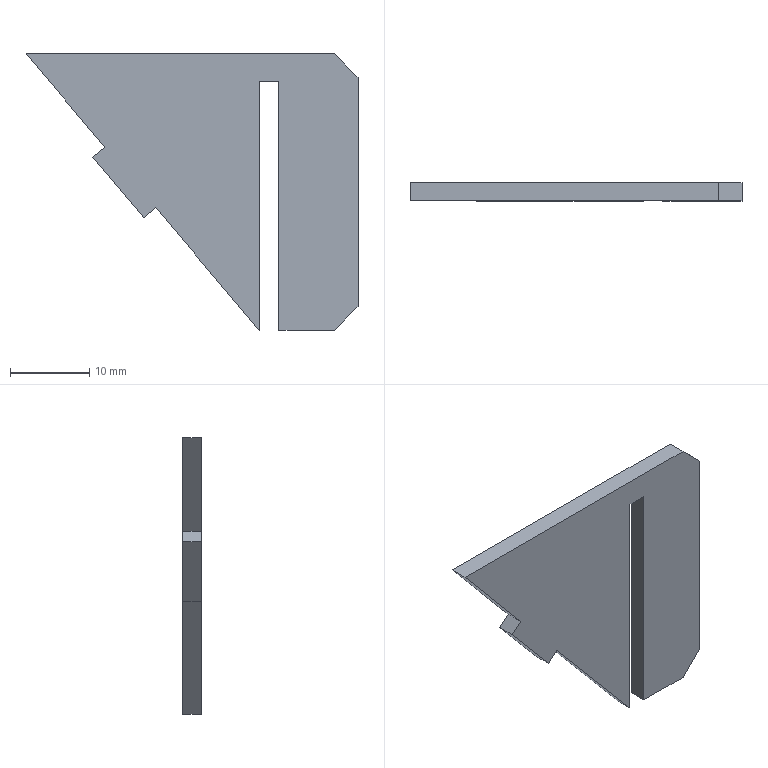Part | SolidWorks | features FlatPattern 1, SMBaseFlange 1, SheetMetal 1 | 1 solid | 15 faces | box 42 x 2.3 x 35 mm | volume 2038 mm3 | plane 15
STEP:
#1=CARTESIAN_POINT('',(9.989,0.,-11.852));
#2=VERTEX_POINT('',#1);
#3=CARTESIAN_POINT('',(0.,0.,0.));
#4=VERTEX_POINT('',#3);
#5=CARTESIAN_POINT('',(9.989,0.,-11.852));
#6=DIRECTION('',(-0.6445,0.,0.7646));
#7=VECTOR('',#6,1000.);
#8=LINE('',#5,#7);
#9=EDGE_CURVE('',#2,#4,#8,.T.);
#10=ORIENTED_EDGE('',*,*,#9,.F.);
#11=CARTESIAN_POINT('',(9.989,-2.3,-11.852));
#12=VERTEX_POINT('',#11);
#13=CARTESIAN_POINT('',(9.989,-2.3,-11.852));
#14=DIRECTION('',(0.,1.,0.));
#15=VECTOR('',#14,1000.);
#16=LINE('',#13,#15);
#17=EDGE_CURVE('',#12,#2,#16,.T.);
#18=ORIENTED_EDGE('',*,*,#17,.F.);
#19=CARTESIAN_POINT('',(0.,-2.3,0.));
#20=VERTEX_POINT('',#19);
#21=CARTESIAN_POINT('',(9.989,-2.3,-11.852));
#22=DIRECTION('',(-0.6445,0.,0.7646));
#23=VECTOR('',#22,1000.);
#24=LINE('',#21,#23);
#25=EDGE_CURVE('',#12,#20,#24,.T.);
#26=ORIENTED_EDGE('',*,*,#25,.T.);
#27=CARTESIAN_POINT('',(0.,-2.3,0.));
#28=DIRECTION('',(0.,1.,0.));
#29=VECTOR('',#28,1000.);
#30=LINE('',#27,#29);
#31=EDGE_CURVE('',#20,#4,#30,.T.);
#32=ORIENTED_EDGE('',*,*,#31,.T.);
#33=EDGE_LOOP('',(#10,#18,#26,#32));
#34=FACE_OUTER_BOUND('',#33,.T.);
#35=CARTESIAN_POINT('',(9.989,-2.3,-11.852));
#36=DIRECTION('',(-0.7646,0.,-0.6445));
#37=DIRECTION('',(-0.6445,0.,0.7646));
#38=AXIS2_PLACEMENT_3D('',#35,#36,#37);
#39=PLANE('',#38);
#40=ADVANCED_FACE('',(#34),#39,.T.);
#41=CARTESIAN_POINT('',(8.46,0.,-13.141));
#42=VERTEX_POINT('',#41);
#43=CARTESIAN_POINT('',(8.46,0.,-13.141));
#44=DIRECTION('',(0.7646,0.,0.6445));
#45=VECTOR('',#44,1000.);
#46=LINE('',#43,#45);
#47=EDGE_CURVE('',#42,#2,#46,.T.);
#48=ORIENTED_EDGE('',*,*,#47,.F.);
#49=CARTESIAN_POINT('',(8.46,-2.3,-13.141));
#50=VERTEX_POINT('',#49);
#51=CARTESIAN_POINT('',(8.46,-2.3,-13.141));
#52=DIRECTION('',(0.,1.,0.));
#53=VECTOR('',#52,1000.);
#54=LINE('',#51,#53);
#55=EDGE_CURVE('',#50,#42,#54,.T.);
#56=ORIENTED_EDGE('',*,*,#55,.F.);
#57=CARTESIAN_POINT('',(8.46,-2.3,-13.141));
#58=DIRECTION('',(0.7646,0.,0.6445));
#59=VECTOR('',#58,1000.);
#60=LINE('',#57,#59);
#61=EDGE_CURVE('',#50,#12,#60,.T.);
#62=ORIENTED_EDGE('',*,*,#61,.T.);
#63=ORIENTED_EDGE('',*,*,#17,.T.);
#64=EDGE_LOOP('',(#48,#56,#62,#63));
#65=FACE_OUTER_BOUND('',#64,.T.);
#66=CARTESIAN_POINT('',(8.46,-2.3,-13.141));
#67=DIRECTION('',(-0.6445,0.,0.7646));
#68=DIRECTION('',(0.7646,0.,0.6445));
#69=AXIS2_PLACEMENT_3D('',#66,#67,#68);
#70=PLANE('',#69);
#71=ADVANCED_FACE('',(#65),#70,.T.);
#72=CARTESIAN_POINT('',(14.905,0.,-20.787));
#73=VERTEX_POINT('',#72);
#74=CARTESIAN_POINT('',(14.905,0.,-20.787));
#75=DIRECTION('',(-0.6445,0.,0.7646));
#76=VECTOR('',#75,1000.);
#77=LINE('',#74,#76);
#78=EDGE_CURVE('',#73,#42,#77,.T.);
#79=ORIENTED_EDGE('',*,*,#78,.F.);
#80=CARTESIAN_POINT('',(14.905,-2.3,-20.787));
#81=VERTEX_POINT('',#80);
#82=CARTESIAN_POINT('',(14.905,-2.3,-20.787));
#83=DIRECTION('',(0.,1.,0.));
#84=VECTOR('',#83,1000.);
#85=LINE('',#82,#84);
#86=EDGE_CURVE('',#81,#73,#85,.T.);
#87=ORIENTED_EDGE('',*,*,#86,.F.);
#88=CARTESIAN_POINT('',(14.905,-2.3,-20.787));
#89=DIRECTION('',(-0.6445,0.,0.7646));
#90=VECTOR('',#89,1000.);
#91=LINE('',#88,#90);
#92=EDGE_CURVE('',#81,#50,#91,.T.);
#93=ORIENTED_EDGE('',*,*,#92,.T.);
#94=ORIENTED_EDGE('',*,*,#55,.T.);
#95=EDGE_LOOP('',(#79,#87,#93,#94));
#96=FACE_OUTER_BOUND('',#95,.T.);
#97=CARTESIAN_POINT('',(14.905,-2.3,-20.787));
#98=DIRECTION('',(-0.7646,0.,-0.6445));
#99=DIRECTION('',(-0.6445,0.,0.7646));
#100=AXIS2_PLACEMENT_3D('',#97,#98,#99);
#101=PLANE('',#100);
#102=ADVANCED_FACE('',(#96),#101,.T.);
#103=CARTESIAN_POINT('',(16.434,0.,-19.498));
#104=VERTEX_POINT('',#103);
#105=CARTESIAN_POINT('',(16.434,0.,-19.498));
#106=DIRECTION('',(-0.7646,0.,-0.6445));
#107=VECTOR('',#106,1000.);
#108=LINE('',#105,#107);
#109=EDGE_CURVE('',#104,#73,#108,.T.);
#110=ORIENTED_EDGE('',*,*,#109,.F.);
#111=CARTESIAN_POINT('',(16.434,-2.3,-19.498));
#112=VERTEX_POINT('',#111);
#113=CARTESIAN_POINT('',(16.434,-2.3,-19.498));
#114=DIRECTION('',(0.,1.,0.));
#115=VECTOR('',#114,1000.);
#116=LINE('',#113,#115);
#117=EDGE_CURVE('',#112,#104,#116,.T.);
#118=ORIENTED_EDGE('',*,*,#117,.F.);
#119=CARTESIAN_POINT('',(16.434,-2.3,-19.498));
#120=DIRECTION('',(-0.7646,0.,-0.6445));
#121=VECTOR('',#120,1000.);
#122=LINE('',#119,#121);
#123=EDGE_CURVE('',#112,#81,#122,.T.);
#124=ORIENTED_EDGE('',*,*,#123,.T.);
#125=ORIENTED_EDGE('',*,*,#86,.T.);
#126=EDGE_LOOP('',(#110,#118,#124,#125));
#127=FACE_OUTER_BOUND('',#126,.T.);
#128=CARTESIAN_POINT('',(16.434,-2.3,-19.498));
#129=DIRECTION('',(0.6445,0.,-0.7646));
#130=DIRECTION('',(-0.7646,0.,-0.6445));
#131=AXIS2_PLACEMENT_3D('',#128,#129,#130);
#132=PLANE('',#131);
#133=ADVANCED_FACE('',(#127),#132,.T.);
#134=CARTESIAN_POINT('',(29.5,0.,-35.));
#135=VERTEX_POINT('',#134);
#136=CARTESIAN_POINT('',(29.5,0.,-35.));
#137=DIRECTION('',(-0.6445,0.,0.7646));
#138=VECTOR('',#137,1000.);
#139=LINE('',#136,#138);
#140=EDGE_CURVE('',#135,#104,#139,.T.);
#141=ORIENTED_EDGE('',*,*,#140,.F.);
#142=CARTESIAN_POINT('',(29.5,-2.3,-35.));
#143=VERTEX_POINT('',#142);
#144=CARTESIAN_POINT('',(29.5,-2.3,-35.));
#145=DIRECTION('',(0.,1.,0.));
#146=VECTOR('',#145,1000.);
#147=LINE('',#144,#146);
#148=EDGE_CURVE('',#143,#135,#147,.T.);
#149=ORIENTED_EDGE('',*,*,#148,.F.);
#150=CARTESIAN_POINT('',(29.5,-2.3,-35.));
#151=DIRECTION('',(-0.6445,0.,0.7646));
#152=VECTOR('',#151,1000.);
#153=LINE('',#150,#152);
#154=EDGE_CURVE('',#143,#112,#153,.T.);
#155=ORIENTED_EDGE('',*,*,#154,.T.);
#156=ORIENTED_EDGE('',*,*,#117,.T.);
#157=EDGE_LOOP('',(#141,#149,#155,#156));
#158=FACE_OUTER_BOUND('',#157,.T.);
#159=CARTESIAN_POINT('',(29.5,-2.3,-35.));
#160=DIRECTION('',(-0.7646,0.,-0.6445));
#161=DIRECTION('',(-0.6445,0.,0.7646));
#162=AXIS2_PLACEMENT_3D('',#159,#160,#161);
#163=PLANE('',#162);
#164=ADVANCED_FACE('',(#158),#163,.T.);
#165=CARTESIAN_POINT('',(29.5,0.,-3.5));
#166=VERTEX_POINT('',#165);
#167=CARTESIAN_POINT('',(29.5,0.,-3.5));
#168=DIRECTION('',(0.,0.,-1.));
#169=VECTOR('',#168,1000.);
#170=LINE('',#167,#169);
#171=EDGE_CURVE('',#166,#135,#170,.T.);
#172=ORIENTED_EDGE('',*,*,#171,.F.);
#173=CARTESIAN_POINT('',(29.5,-2.3,-3.5));
#174=VERTEX_POINT('',#173);
#175=CARTESIAN_POINT('',(29.5,-2.3,-3.5));
#176=DIRECTION('',(0.,1.,0.));
#177=VECTOR('',#176,1000.);
#178=LINE('',#175,#177);
#179=EDGE_CURVE('',#174,#166,#178,.T.);
#180=ORIENTED_EDGE('',*,*,#179,.F.);
#181=CARTESIAN_POINT('',(29.5,-2.3,-3.5));
#182=DIRECTION('',(0.,0.,-1.));
#183=VECTOR('',#182,1000.);
#184=LINE('',#181,#183);
#185=EDGE_CURVE('',#174,#143,#184,.T.);
#186=ORIENTED_EDGE('',*,*,#185,.T.);
#187=ORIENTED_EDGE('',*,*,#148,.T.);
#188=EDGE_LOOP('',(#172,#180,#186,#187));
#189=FACE_OUTER_BOUND('',#188,.T.);
#190=CARTESIAN_POINT('',(29.5,-2.3,-3.5));
#191=DIRECTION('',(1.,0.,0.));
#192=DIRECTION('',(0.,0.,-1.));
#193=AXIS2_PLACEMENT_3D('',#190,#191,#192);
#194=PLANE('',#193);
#195=ADVANCED_FACE('',(#189),#194,.T.);
#196=CARTESIAN_POINT('',(32.,0.,-3.5));
#197=VERTEX_POINT('',#196);
#198=CARTESIAN_POINT('',(32.,0.,-3.5));
#199=DIRECTION('',(-1.,0.,0.));
#200=VECTOR('',#199,1000.);
#201=LINE('',#198,#200);
#202=EDGE_CURVE('',#197,#166,#201,.T.);
#203=ORIENTED_EDGE('',*,*,#202,.F.);
#204=CARTESIAN_POINT('',(32.,-2.3,-3.5));
#205=VERTEX_POINT('',#204);
#206=CARTESIAN_POINT('',(32.,-2.3,-3.5));
#207=DIRECTION('',(0.,1.,0.));
#208=VECTOR('',#207,1000.);
#209=LINE('',#206,#208);
#210=EDGE_CURVE('',#205,#197,#209,.T.);
#211=ORIENTED_EDGE('',*,*,#210,.F.);
#212=CARTESIAN_POINT('',(32.,-2.3,-3.5));
#213=DIRECTION('',(-1.,0.,0.));
#214=VECTOR('',#213,1000.);
#215=LINE('',#212,#214);
#216=EDGE_CURVE('',#205,#174,#215,.T.);
#217=ORIENTED_EDGE('',*,*,#216,.T.);
#218=ORIENTED_EDGE('',*,*,#179,.T.);
#219=EDGE_LOOP('',(#203,#211,#217,#218));
#220=FACE_OUTER_BOUND('',#219,.T.);
#221=CARTESIAN_POINT('',(32.,-2.3,-3.5));
#222=DIRECTION('',(0.,0.,-1.));
#223=DIRECTION('',(-1.,0.,0.));
#224=AXIS2_PLACEMENT_3D('',#221,#222,#223);
#225=PLANE('',#224);
#226=ADVANCED_FACE('',(#220),#225,.T.);
#227=CARTESIAN_POINT('',(32.,0.,-35.));
#228=VERTEX_POINT('',#227);
#229=CARTESIAN_POINT('',(32.,0.,-35.));
#230=DIRECTION('',(0.,0.,1.));
#231=VECTOR('',#230,1000.);
#232=LINE('',#229,#231);
#233=EDGE_CURVE('',#228,#197,#232,.T.);
#234=ORIENTED_EDGE('',*,*,#233,.F.);
#235=CARTESIAN_POINT('',(32.,-2.3,-35.));
#236=VERTEX_POINT('',#235);
#237=CARTESIAN_POINT('',(32.,-2.3,-35.));
#238=DIRECTION('',(0.,1.,0.));
#239=VECTOR('',#238,1000.);
#240=LINE('',#237,#239);
#241=EDGE_CURVE('',#236,#228,#240,.T.);
#242=ORIENTED_EDGE('',*,*,#241,.F.);
#243=CARTESIAN_POINT('',(32.,-2.3,-35.));
#244=DIRECTION('',(0.,0.,1.));
#245=VECTOR('',#244,1000.);
#246=LINE('',#243,#245);
#247=EDGE_CURVE('',#236,#205,#246,.T.);
#248=ORIENTED_EDGE('',*,*,#247,.T.);
#249=ORIENTED_EDGE('',*,*,#210,.T.);
#250=EDGE_LOOP('',(#234,#242,#248,#249));
#251=FACE_OUTER_BOUND('',#250,.T.);
#252=CARTESIAN_POINT('',(32.,-2.3,-35.));
#253=DIRECTION('',(-1.,0.,0.));
#254=DIRECTION('',(0.,0.,1.));
#255=AXIS2_PLACEMENT_3D('',#252,#253,#254);
#256=PLANE('',#255);
#257=ADVANCED_FACE('',(#251),#256,.T.);
#258=CARTESIAN_POINT('',(39.,0.,-35.));
#259=VERTEX_POINT('',#258);
#260=CARTESIAN_POINT('',(39.,0.,-35.));
#261=DIRECTION('',(-1.,0.,0.));
#262=VECTOR('',#261,1000.);
#263=LINE('',#260,#262);
#264=EDGE_CURVE('',#259,#228,#263,.T.);
#265=ORIENTED_EDGE('',*,*,#264,.F.);
#266=CARTESIAN_POINT('',(39.,-2.3,-35.));
#267=VERTEX_POINT('',#266);
#268=CARTESIAN_POINT('',(39.,-2.3,-35.));
#269=DIRECTION('',(0.,1.,0.));
#270=VECTOR('',#269,1000.);
#271=LINE('',#268,#270);
#272=EDGE_CURVE('',#267,#259,#271,.T.);
#273=ORIENTED_EDGE('',*,*,#272,.F.);
#274=CARTESIAN_POINT('',(39.,-2.3,-35.));
#275=DIRECTION('',(-1.,0.,0.));
#276=VECTOR('',#275,1000.);
#277=LINE('',#274,#276);
#278=EDGE_CURVE('',#267,#236,#277,.T.);
#279=ORIENTED_EDGE('',*,*,#278,.T.);
#280=ORIENTED_EDGE('',*,*,#241,.T.);
#281=EDGE_LOOP('',(#265,#273,#279,#280));
#282=FACE_OUTER_BOUND('',#281,.T.);
#283=CARTESIAN_POINT('',(39.,-2.3,-35.));
#284=DIRECTION('',(0.,0.,-1.));
#285=DIRECTION('',(-1.,0.,0.));
#286=AXIS2_PLACEMENT_3D('',#283,#284,#285);
#287=PLANE('',#286);
#288=ADVANCED_FACE('',(#282),#287,.T.);
#289=CARTESIAN_POINT('',(42.,0.,-32.));
#290=VERTEX_POINT('',#289);
#291=CARTESIAN_POINT('',(42.,0.,-32.));
#292=DIRECTION('',(-0.7071,0.,-0.7071));
#293=VECTOR('',#292,1000.);
#294=LINE('',#291,#293);
#295=EDGE_CURVE('',#290,#259,#294,.T.);
#296=ORIENTED_EDGE('',*,*,#295,.F.);
#297=CARTESIAN_POINT('',(42.,-2.3,-32.));
#298=VERTEX_POINT('',#297);
#299=CARTESIAN_POINT('',(42.,-2.3,-32.));
#300=DIRECTION('',(0.,1.,0.));
#301=VECTOR('',#300,1000.);
#302=LINE('',#299,#301);
#303=EDGE_CURVE('',#298,#290,#302,.T.);
#304=ORIENTED_EDGE('',*,*,#303,.F.);
#305=CARTESIAN_POINT('',(42.,-2.3,-32.));
#306=DIRECTION('',(-0.7071,0.,-0.7071));
#307=VECTOR('',#306,1000.);
#308=LINE('',#305,#307);
#309=EDGE_CURVE('',#298,#267,#308,.T.);
#310=ORIENTED_EDGE('',*,*,#309,.T.);
#311=ORIENTED_EDGE('',*,*,#272,.T.);
#312=EDGE_LOOP('',(#296,#304,#310,#311));
#313=FACE_OUTER_BOUND('',#312,.T.);
#314=CARTESIAN_POINT('',(42.,-2.3,-32.));
#315=DIRECTION('',(0.7071,0.,-0.7071));
#316=DIRECTION('',(-0.7071,0.,-0.7071));
#317=AXIS2_PLACEMENT_3D('',#314,#315,#316);
#318=PLANE('',#317);
#319=ADVANCED_FACE('',(#313),#318,.T.);
#320=CARTESIAN_POINT('',(42.,0.,-3.));
#321=VERTEX_POINT('',#320);
#322=CARTESIAN_POINT('',(42.,0.,-3.));
#323=DIRECTION('',(0.,0.,-1.));
#324=VECTOR('',#323,1000.);
#325=LINE('',#322,#324);
#326=EDGE_CURVE('',#321,#290,#325,.T.);
#327=ORIENTED_EDGE('',*,*,#326,.F.);
#328=CARTESIAN_POINT('',(42.,-2.3,-3.));
#329=VERTEX_POINT('',#328);
#330=CARTESIAN_POINT('',(42.,-2.3,-3.));
#331=DIRECTION('',(0.,1.,0.));
#332=VECTOR('',#331,1000.);
#333=LINE('',#330,#332);
#334=EDGE_CURVE('',#329,#321,#333,.T.);
#335=ORIENTED_EDGE('',*,*,#334,.F.);
#336=CARTESIAN_POINT('',(42.,-2.3,-3.));
#337=DIRECTION('',(0.,0.,-1.));
#338=VECTOR('',#337,1000.);
#339=LINE('',#336,#338);
#340=EDGE_CURVE('',#329,#298,#339,.T.);
#341=ORIENTED_EDGE('',*,*,#340,.T.);
#342=ORIENTED_EDGE('',*,*,#303,.T.);
#343=EDGE_LOOP('',(#327,#335,#341,#342));
#344=FACE_OUTER_BOUND('',#343,.T.);
#345=CARTESIAN_POINT('',(42.,-2.3,-3.));
#346=DIRECTION('',(1.,0.,0.));
#347=DIRECTION('',(0.,0.,-1.));
#348=AXIS2_PLACEMENT_3D('',#345,#346,#347);
#349=PLANE('',#348);
#350=ADVANCED_FACE('',(#344),#349,.T.);
#351=CARTESIAN_POINT('',(39.,0.,0.));
#352=VERTEX_POINT('',#351);
#353=CARTESIAN_POINT('',(39.,0.,0.));
#354=DIRECTION('',(0.7071,0.,-0.7071));
#355=VECTOR('',#354,1000.);
#356=LINE('',#353,#355);
#357=EDGE_CURVE('',#352,#321,#356,.T.);
#358=ORIENTED_EDGE('',*,*,#357,.F.);
#359=CARTESIAN_POINT('',(39.,-2.3,0.));
#360=VERTEX_POINT('',#359);
#361=CARTESIAN_POINT('',(39.,-2.3,0.));
#362=DIRECTION('',(0.,1.,0.));
#363=VECTOR('',#362,1000.);
#364=LINE('',#361,#363);
#365=EDGE_CURVE('',#360,#352,#364,.T.);
#366=ORIENTED_EDGE('',*,*,#365,.F.);
#367=CARTESIAN_POINT('',(39.,-2.3,0.));
#368=DIRECTION('',(0.7071,0.,-0.7071));
#369=VECTOR('',#368,1000.);
#370=LINE('',#367,#369);
#371=EDGE_CURVE('',#360,#329,#370,.T.);
#372=ORIENTED_EDGE('',*,*,#371,.T.);
#373=ORIENTED_EDGE('',*,*,#334,.T.);
#374=EDGE_LOOP('',(#358,#366,#372,#373));
#375=FACE_OUTER_BOUND('',#374,.T.);
#376=CARTESIAN_POINT('',(39.,-2.3,0.));
#377=DIRECTION('',(0.7071,0.,0.7071));
#378=DIRECTION('',(0.7071,0.,-0.7071));
#379=AXIS2_PLACEMENT_3D('',#376,#377,#378);
#380=PLANE('',#379);
#381=ADVANCED_FACE('',(#375),#380,.T.);
#382=CARTESIAN_POINT('',(0.,0.,0.));
#383=DIRECTION('',(1.,0.,0.));
#384=VECTOR('',#383,1000.);
#385=LINE('',#382,#384);
#386=EDGE_CURVE('',#4,#352,#385,.T.);
#387=ORIENTED_EDGE('',*,*,#386,.F.);
#388=ORIENTED_EDGE('',*,*,#31,.F.);
#389=CARTESIAN_POINT('',(0.,-2.3,0.));
#390=DIRECTION('',(1.,0.,0.));
#391=VECTOR('',#390,1000.);
#392=LINE('',#389,#391);
#393=EDGE_CURVE('',#20,#360,#392,.T.);
#394=ORIENTED_EDGE('',*,*,#393,.T.);
#395=ORIENTED_EDGE('',*,*,#365,.T.);
#396=EDGE_LOOP('',(#387,#388,#394,#395));
#397=FACE_OUTER_BOUND('',#396,.T.);
#398=CARTESIAN_POINT('',(0.,-2.3,0.));
#399=DIRECTION('',(0.,0.,1.));
#400=DIRECTION('',(1.,0.,0.));
#401=AXIS2_PLACEMENT_3D('',#398,#399,#400);
#402=PLANE('',#401);
#403=ADVANCED_FACE('',(#397),#402,.T.);
#404=ORIENTED_EDGE('',*,*,#25,.F.);
#405=ORIENTED_EDGE('',*,*,#61,.F.);
#406=ORIENTED_EDGE('',*,*,#92,.F.);
#407=ORIENTED_EDGE('',*,*,#123,.F.);
#408=ORIENTED_EDGE('',*,*,#154,.F.);
#409=ORIENTED_EDGE('',*,*,#185,.F.);
#410=ORIENTED_EDGE('',*,*,#216,.F.);
#411=ORIENTED_EDGE('',*,*,#247,.F.);
#412=ORIENTED_EDGE('',*,*,#278,.F.);
#413=ORIENTED_EDGE('',*,*,#309,.F.);
#414=ORIENTED_EDGE('',*,*,#340,.F.);
#415=ORIENTED_EDGE('',*,*,#371,.F.);
#416=ORIENTED_EDGE('',*,*,#393,.F.);
#417=EDGE_LOOP('',(#404,#405,#406,#407,#408,#409,#410,#411,#412,#413,#414,#415,#416));
#418=FACE_OUTER_BOUND('',#417,.T.);
#419=CARTESIAN_POINT('',(0.,-2.3,0.));
#420=DIRECTION('',(0.,-1.,0.));
#421=DIRECTION('',(0.,0.,-1.));
#422=AXIS2_PLACEMENT_3D('',#419,#420,#421);
#423=PLANE('',#422);
#424=ADVANCED_FACE('',(#418),#423,.T.);
#425=ORIENTED_EDGE('',*,*,#9,.T.);
#426=ORIENTED_EDGE('',*,*,#386,.T.);
#427=ORIENTED_EDGE('',*,*,#357,.T.);
#428=ORIENTED_EDGE('',*,*,#326,.T.);
#429=ORIENTED_EDGE('',*,*,#295,.T.);
#430=ORIENTED_EDGE('',*,*,#264,.T.);
#431=ORIENTED_EDGE('',*,*,#233,.T.);
#432=ORIENTED_EDGE('',*,*,#202,.T.);
#433=ORIENTED_EDGE('',*,*,#171,.T.);
#434=ORIENTED_EDGE('',*,*,#140,.T.);
#435=ORIENTED_EDGE('',*,*,#109,.T.);
#436=ORIENTED_EDGE('',*,*,#78,.T.);
#437=ORIENTED_EDGE('',*,*,#47,.T.);
#438=EDGE_LOOP('',(#425,#426,#427,#428,#429,#430,#431,#432,#433,#434,#435,#436,#437));
#439=FACE_OUTER_BOUND('',#438,.T.);
#440=CARTESIAN_POINT('',(0.,0.,0.));
#441=DIRECTION('',(0.,-1.,0.));
#442=DIRECTION('',(0.,0.,-1.));
#443=AXIS2_PLACEMENT_3D('',#440,#441,#442);
#444=PLANE('',#443);
#445=ADVANCED_FACE('',(#439),#444,.F.);
#446=CLOSED_SHELL('',(#40,#71,#102,#133,#164,#195,#226,#257,#288,#319,#350,#381,#403,#424,#445));
#447=MANIFOLD_SOLID_BREP('',#446);
#448=CARTESIAN_POINT('',(0.,0.,0.));
#449=DIRECTION('',(0.,0.,1.));
#450=DIRECTION('',(1.,0.,0.));
#451=AXIS2_PLACEMENT_3D('',#448,#449,#450);
#452=(LENGTH_UNIT()NAMED_UNIT(*)SI_UNIT(.MILLI.,.METRE.));
#453=UNCERTAINTY_MEASURE_WITH_UNIT(LENGTH_MEASURE(0.00001),#452,'','');
#454=(NAMED_UNIT(*)PLANE_ANGLE_UNIT()SI_UNIT($,.RADIAN.));
#455=(NAMED_UNIT(*)SI_UNIT($,.STERADIAN.)SOLID_ANGLE_UNIT());
#456=(GEOMETRIC_REPRESENTATION_CONTEXT(3)GLOBAL_UNCERTAINTY_ASSIGNED_CONTEXT((#453))GLOBAL_UNIT_ASSIGNED_CONTEXT((#452,#454,#455))REPRESENTATION_CONTEXT('',''));
#457=ADVANCED_BREP_SHAPE_REPRESENTATION('',(#447,#451),#456);